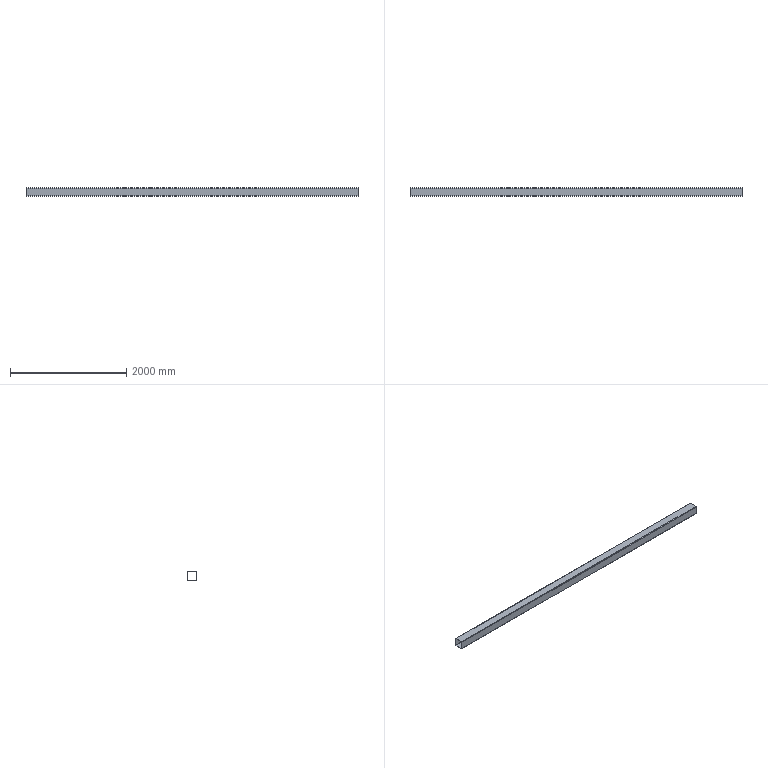Part | SolidWorks | features WeldMemberFeat 1, WeldmentFeature 1 | 1 solid | 18 faces | box 5700 x 150 x 150 mm | volume 16163031 mm3 | plane 10 | cylinder 8 | commonest cylinder face diameters 10 x4 20 x4
STEP:
#1=CARTESIAN_POINT('',(-2850.,75.,65.));
#2=VERTEX_POINT('',#1);
#3=CARTESIAN_POINT('',(-2850.,65.,75.));
#4=VERTEX_POINT('',#3);
#5=CARTESIAN_POINT('',(-2850.,65.,65.));
#6=DIRECTION('',(1.,0.,0.));
#7=DIRECTION('',(0.,1.,0.));
#8=AXIS2_PLACEMENT_3D('',#5,#6,#7);
#9=CIRCLE('',#8,10.);
#10=EDGE_CURVE('',#2,#4,#9,.T.);
#11=ORIENTED_EDGE('',*,*,#10,.T.);
#12=CARTESIAN_POINT('',(2850.,65.,75.));
#13=VERTEX_POINT('',#12);
#14=CARTESIAN_POINT('',(2850.,65.,75.));
#15=DIRECTION('',(-1.,0.,0.));
#16=VECTOR('',#15,1000.);
#17=LINE('',#14,#16);
#18=EDGE_CURVE('',#13,#4,#17,.T.);
#19=ORIENTED_EDGE('',*,*,#18,.F.);
#20=CARTESIAN_POINT('',(2850.,75.,65.));
#21=VERTEX_POINT('',#20);
#22=CARTESIAN_POINT('',(2850.,65.,65.));
#23=DIRECTION('',(1.,0.,0.));
#24=DIRECTION('',(0.,1.,0.));
#25=AXIS2_PLACEMENT_3D('',#22,#23,#24);
#26=CIRCLE('',#25,10.);
#27=EDGE_CURVE('',#21,#13,#26,.T.);
#28=ORIENTED_EDGE('',*,*,#27,.F.);
#29=CARTESIAN_POINT('',(2850.,75.,65.));
#30=DIRECTION('',(-1.,0.,0.));
#31=VECTOR('',#30,1000.);
#32=LINE('',#29,#31);
#33=EDGE_CURVE('',#21,#2,#32,.T.);
#34=ORIENTED_EDGE('',*,*,#33,.T.);
#35=EDGE_LOOP('',(#11,#19,#28,#34));
#36=FACE_OUTER_BOUND('',#35,.T.);
#37=CARTESIAN_POINT('',(2850.,65.,65.));
#38=DIRECTION('',(-1.,0.,0.));
#39=DIRECTION('',(0.,-1.,0.));
#40=AXIS2_PLACEMENT_3D('',#37,#38,#39);
#41=CYLINDRICAL_SURFACE('',#40,10.);
#42=ADVANCED_FACE('',(#36),#41,.T.);
#43=CARTESIAN_POINT('',(-2850.,-65.,75.));
#44=VERTEX_POINT('',#43);
#45=CARTESIAN_POINT('',(-2850.,65.,75.));
#46=DIRECTION('',(0.,-1.,0.));
#47=VECTOR('',#46,1000.);
#48=LINE('',#45,#47);
#49=EDGE_CURVE('',#4,#44,#48,.T.);
#50=ORIENTED_EDGE('',*,*,#49,.T.);
#51=CARTESIAN_POINT('',(2850.,-65.,75.));
#52=VERTEX_POINT('',#51);
#53=CARTESIAN_POINT('',(2850.,-65.,75.));
#54=DIRECTION('',(-1.,0.,0.));
#55=VECTOR('',#54,1000.);
#56=LINE('',#53,#55);
#57=EDGE_CURVE('',#52,#44,#56,.T.);
#58=ORIENTED_EDGE('',*,*,#57,.F.);
#59=CARTESIAN_POINT('',(2850.,65.,75.));
#60=DIRECTION('',(0.,-1.,0.));
#61=VECTOR('',#60,1000.);
#62=LINE('',#59,#61);
#63=EDGE_CURVE('',#13,#52,#62,.T.);
#64=ORIENTED_EDGE('',*,*,#63,.F.);
#65=ORIENTED_EDGE('',*,*,#18,.T.);
#66=EDGE_LOOP('',(#50,#58,#64,#65));
#67=FACE_OUTER_BOUND('',#66,.T.);
#68=CARTESIAN_POINT('',(2850.,65.,75.));
#69=DIRECTION('',(0.,0.,-1.));
#70=DIRECTION('',(-1.,0.,0.));
#71=AXIS2_PLACEMENT_3D('',#68,#69,#70);
#72=PLANE('',#71);
#73=ADVANCED_FACE('',(#67),#72,.F.);
#74=CARTESIAN_POINT('',(-2850.,-75.,65.));
#75=VERTEX_POINT('',#74);
#76=CARTESIAN_POINT('',(-2850.,-65.,65.));
#77=DIRECTION('',(1.,0.,0.));
#78=DIRECTION('',(0.,1.,0.));
#79=AXIS2_PLACEMENT_3D('',#76,#77,#78);
#80=CIRCLE('',#79,10.);
#81=EDGE_CURVE('',#44,#75,#80,.T.);
#82=ORIENTED_EDGE('',*,*,#81,.T.);
#83=CARTESIAN_POINT('',(2850.,-75.,65.));
#84=VERTEX_POINT('',#83);
#85=CARTESIAN_POINT('',(2850.,-75.,65.));
#86=DIRECTION('',(-1.,0.,0.));
#87=VECTOR('',#86,1000.);
#88=LINE('',#85,#87);
#89=EDGE_CURVE('',#84,#75,#88,.T.);
#90=ORIENTED_EDGE('',*,*,#89,.F.);
#91=CARTESIAN_POINT('',(2850.,-65.,65.));
#92=DIRECTION('',(1.,0.,0.));
#93=DIRECTION('',(0.,1.,0.));
#94=AXIS2_PLACEMENT_3D('',#91,#92,#93);
#95=CIRCLE('',#94,10.);
#96=EDGE_CURVE('',#52,#84,#95,.T.);
#97=ORIENTED_EDGE('',*,*,#96,.F.);
#98=ORIENTED_EDGE('',*,*,#57,.T.);
#99=EDGE_LOOP('',(#82,#90,#97,#98));
#100=FACE_OUTER_BOUND('',#99,.T.);
#101=CARTESIAN_POINT('',(2850.,-65.,65.));
#102=DIRECTION('',(-1.,0.,0.));
#103=DIRECTION('',(0.,-1.,0.));
#104=AXIS2_PLACEMENT_3D('',#101,#102,#103);
#105=CYLINDRICAL_SURFACE('',#104,10.);
#106=ADVANCED_FACE('',(#100),#105,.T.);
#107=CARTESIAN_POINT('',(-2850.,-75.,-65.));
#108=VERTEX_POINT('',#107);
#109=CARTESIAN_POINT('',(-2850.,-75.,-65.));
#110=DIRECTION('',(0.,0.,-1.));
#111=VECTOR('',#110,1000.);
#112=LINE('',#109,#111);
#113=EDGE_CURVE('',#75,#108,#112,.T.);
#114=ORIENTED_EDGE('',*,*,#113,.T.);
#115=CARTESIAN_POINT('',(2850.,-75.,-65.));
#116=VERTEX_POINT('',#115);
#117=CARTESIAN_POINT('',(2850.,-75.,-65.));
#118=DIRECTION('',(-1.,0.,0.));
#119=VECTOR('',#118,1000.);
#120=LINE('',#117,#119);
#121=EDGE_CURVE('',#116,#108,#120,.T.);
#122=ORIENTED_EDGE('',*,*,#121,.F.);
#123=CARTESIAN_POINT('',(2850.,-75.,-65.));
#124=DIRECTION('',(0.,0.,-1.));
#125=VECTOR('',#124,1000.);
#126=LINE('',#123,#125);
#127=EDGE_CURVE('',#84,#116,#126,.T.);
#128=ORIENTED_EDGE('',*,*,#127,.F.);
#129=ORIENTED_EDGE('',*,*,#89,.T.);
#130=EDGE_LOOP('',(#114,#122,#128,#129));
#131=FACE_OUTER_BOUND('',#130,.T.);
#132=CARTESIAN_POINT('',(2850.,-75.,-65.));
#133=DIRECTION('',(0.,1.,0.));
#134=DIRECTION('',(-1.,0.,0.));
#135=AXIS2_PLACEMENT_3D('',#132,#133,#134);
#136=PLANE('',#135);
#137=ADVANCED_FACE('',(#131),#136,.F.);
#138=CARTESIAN_POINT('',(-2850.,-65.,-75.));
#139=VERTEX_POINT('',#138);
#140=CARTESIAN_POINT('',(-2850.,-65.,-65.));
#141=DIRECTION('',(1.,0.,0.));
#142=DIRECTION('',(0.,1.,0.));
#143=AXIS2_PLACEMENT_3D('',#140,#141,#142);
#144=CIRCLE('',#143,10.);
#145=EDGE_CURVE('',#108,#139,#144,.T.);
#146=ORIENTED_EDGE('',*,*,#145,.T.);
#147=CARTESIAN_POINT('',(2850.,-65.,-75.));
#148=VERTEX_POINT('',#147);
#149=CARTESIAN_POINT('',(2850.,-65.,-75.));
#150=DIRECTION('',(-1.,0.,0.));
#151=VECTOR('',#150,1000.);
#152=LINE('',#149,#151);
#153=EDGE_CURVE('',#148,#139,#152,.T.);
#154=ORIENTED_EDGE('',*,*,#153,.F.);
#155=CARTESIAN_POINT('',(2850.,-65.,-65.));
#156=DIRECTION('',(1.,0.,0.));
#157=DIRECTION('',(0.,1.,0.));
#158=AXIS2_PLACEMENT_3D('',#155,#156,#157);
#159=CIRCLE('',#158,10.);
#160=EDGE_CURVE('',#116,#148,#159,.T.);
#161=ORIENTED_EDGE('',*,*,#160,.F.);
#162=ORIENTED_EDGE('',*,*,#121,.T.);
#163=EDGE_LOOP('',(#146,#154,#161,#162));
#164=FACE_OUTER_BOUND('',#163,.T.);
#165=CARTESIAN_POINT('',(2850.,-65.,-65.));
#166=DIRECTION('',(-1.,0.,0.));
#167=DIRECTION('',(0.,-1.,0.));
#168=AXIS2_PLACEMENT_3D('',#165,#166,#167);
#169=CYLINDRICAL_SURFACE('',#168,10.);
#170=ADVANCED_FACE('',(#164),#169,.T.);
#171=CARTESIAN_POINT('',(-2850.,65.,-75.));
#172=VERTEX_POINT('',#171);
#173=CARTESIAN_POINT('',(-2850.,-65.,-75.));
#174=DIRECTION('',(0.,1.,0.));
#175=VECTOR('',#174,1000.);
#176=LINE('',#173,#175);
#177=EDGE_CURVE('',#139,#172,#176,.T.);
#178=ORIENTED_EDGE('',*,*,#177,.T.);
#179=CARTESIAN_POINT('',(2850.,65.,-75.));
#180=VERTEX_POINT('',#179);
#181=CARTESIAN_POINT('',(2850.,65.,-75.));
#182=DIRECTION('',(-1.,0.,0.));
#183=VECTOR('',#182,1000.);
#184=LINE('',#181,#183);
#185=EDGE_CURVE('',#180,#172,#184,.T.);
#186=ORIENTED_EDGE('',*,*,#185,.F.);
#187=CARTESIAN_POINT('',(2850.,-65.,-75.));
#188=DIRECTION('',(0.,1.,0.));
#189=VECTOR('',#188,1000.);
#190=LINE('',#187,#189);
#191=EDGE_CURVE('',#148,#180,#190,.T.);
#192=ORIENTED_EDGE('',*,*,#191,.F.);
#193=ORIENTED_EDGE('',*,*,#153,.T.);
#194=EDGE_LOOP('',(#178,#186,#192,#193));
#195=FACE_OUTER_BOUND('',#194,.T.);
#196=CARTESIAN_POINT('',(2850.,-65.,-75.));
#197=DIRECTION('',(0.,0.,1.));
#198=DIRECTION('',(1.,0.,0.));
#199=AXIS2_PLACEMENT_3D('',#196,#197,#198);
#200=PLANE('',#199);
#201=ADVANCED_FACE('',(#195),#200,.F.);
#202=CARTESIAN_POINT('',(-2850.,75.,-65.));
#203=VERTEX_POINT('',#202);
#204=CARTESIAN_POINT('',(-2850.,65.,-65.));
#205=DIRECTION('',(1.,0.,0.));
#206=DIRECTION('',(0.,1.,0.));
#207=AXIS2_PLACEMENT_3D('',#204,#205,#206);
#208=CIRCLE('',#207,10.);
#209=EDGE_CURVE('',#172,#203,#208,.T.);
#210=ORIENTED_EDGE('',*,*,#209,.T.);
#211=CARTESIAN_POINT('',(2850.,75.,-65.));
#212=VERTEX_POINT('',#211);
#213=CARTESIAN_POINT('',(2850.,75.,-65.));
#214=DIRECTION('',(-1.,0.,0.));
#215=VECTOR('',#214,1000.);
#216=LINE('',#213,#215);
#217=EDGE_CURVE('',#212,#203,#216,.T.);
#218=ORIENTED_EDGE('',*,*,#217,.F.);
#219=CARTESIAN_POINT('',(2850.,65.,-65.));
#220=DIRECTION('',(1.,0.,0.));
#221=DIRECTION('',(0.,1.,0.));
#222=AXIS2_PLACEMENT_3D('',#219,#220,#221);
#223=CIRCLE('',#222,10.);
#224=EDGE_CURVE('',#180,#212,#223,.T.);
#225=ORIENTED_EDGE('',*,*,#224,.F.);
#226=ORIENTED_EDGE('',*,*,#185,.T.);
#227=EDGE_LOOP('',(#210,#218,#225,#226));
#228=FACE_OUTER_BOUND('',#227,.T.);
#229=CARTESIAN_POINT('',(2850.,65.,-65.));
#230=DIRECTION('',(-1.,0.,0.));
#231=DIRECTION('',(0.,-1.,0.));
#232=AXIS2_PLACEMENT_3D('',#229,#230,#231);
#233=CYLINDRICAL_SURFACE('',#232,10.);
#234=ADVANCED_FACE('',(#228),#233,.T.);
#235=CARTESIAN_POINT('',(-2850.,-65.,70.));
#236=VERTEX_POINT('',#235);
#237=CARTESIAN_POINT('',(-2850.,-70.,65.));
#238=VERTEX_POINT('',#237);
#239=CARTESIAN_POINT('',(-2850.,-65.,65.));
#240=DIRECTION('',(1.,0.,0.));
#241=DIRECTION('',(0.,1.,0.));
#242=AXIS2_PLACEMENT_3D('',#239,#240,#241);
#243=CIRCLE('',#242,5.);
#244=EDGE_CURVE('',#236,#238,#243,.T.);
#245=ORIENTED_EDGE('',*,*,#244,.F.);
#246=CARTESIAN_POINT('',(2850.,-65.,70.));
#247=VERTEX_POINT('',#246);
#248=CARTESIAN_POINT('',(2850.,-65.,70.));
#249=DIRECTION('',(-1.,0.,0.));
#250=VECTOR('',#249,1000.);
#251=LINE('',#248,#250);
#252=EDGE_CURVE('',#247,#236,#251,.T.);
#253=ORIENTED_EDGE('',*,*,#252,.F.);
#254=CARTESIAN_POINT('',(2850.,-70.,65.));
#255=VERTEX_POINT('',#254);
#256=CARTESIAN_POINT('',(2850.,-65.,65.));
#257=DIRECTION('',(1.,0.,0.));
#258=DIRECTION('',(0.,1.,0.));
#259=AXIS2_PLACEMENT_3D('',#256,#257,#258);
#260=CIRCLE('',#259,5.);
#261=EDGE_CURVE('',#247,#255,#260,.T.);
#262=ORIENTED_EDGE('',*,*,#261,.T.);
#263=CARTESIAN_POINT('',(2850.,-70.,65.));
#264=DIRECTION('',(-1.,0.,0.));
#265=VECTOR('',#264,1000.);
#266=LINE('',#263,#265);
#267=EDGE_CURVE('',#255,#238,#266,.T.);
#268=ORIENTED_EDGE('',*,*,#267,.T.);
#269=EDGE_LOOP('',(#245,#253,#262,#268));
#270=FACE_OUTER_BOUND('',#269,.T.);
#271=CARTESIAN_POINT('',(2850.,-65.,65.));
#272=DIRECTION('',(-1.,0.,0.));
#273=DIRECTION('',(0.,-1.,0.));
#274=AXIS2_PLACEMENT_3D('',#271,#272,#273);
#275=CYLINDRICAL_SURFACE('',#274,5.);
#276=ADVANCED_FACE('',(#270),#275,.F.);
#277=CARTESIAN_POINT('',(-2850.,65.,70.));
#278=VERTEX_POINT('',#277);
#279=CARTESIAN_POINT('',(-2850.,65.,70.));
#280=DIRECTION('',(0.,-1.,0.));
#281=VECTOR('',#280,1000.);
#282=LINE('',#279,#281);
#283=EDGE_CURVE('',#278,#236,#282,.T.);
#284=ORIENTED_EDGE('',*,*,#283,.F.);
#285=CARTESIAN_POINT('',(2850.,65.,70.));
#286=VERTEX_POINT('',#285);
#287=CARTESIAN_POINT('',(2850.,65.,70.));
#288=DIRECTION('',(-1.,0.,0.));
#289=VECTOR('',#288,1000.);
#290=LINE('',#287,#289);
#291=EDGE_CURVE('',#286,#278,#290,.T.);
#292=ORIENTED_EDGE('',*,*,#291,.F.);
#293=CARTESIAN_POINT('',(2850.,65.,70.));
#294=DIRECTION('',(0.,-1.,0.));
#295=VECTOR('',#294,1000.);
#296=LINE('',#293,#295);
#297=EDGE_CURVE('',#286,#247,#296,.T.);
#298=ORIENTED_EDGE('',*,*,#297,.T.);
#299=ORIENTED_EDGE('',*,*,#252,.T.);
#300=EDGE_LOOP('',(#284,#292,#298,#299));
#301=FACE_OUTER_BOUND('',#300,.T.);
#302=CARTESIAN_POINT('',(2850.,65.,70.));
#303=DIRECTION('',(0.,0.,-1.));
#304=DIRECTION('',(-1.,0.,0.));
#305=AXIS2_PLACEMENT_3D('',#302,#303,#304);
#306=PLANE('',#305);
#307=ADVANCED_FACE('',(#301),#306,.T.);
#308=CARTESIAN_POINT('',(-2850.,70.,65.));
#309=VERTEX_POINT('',#308);
#310=CARTESIAN_POINT('',(-2850.,65.,65.));
#311=DIRECTION('',(1.,0.,0.));
#312=DIRECTION('',(0.,1.,0.));
#313=AXIS2_PLACEMENT_3D('',#310,#311,#312);
#314=CIRCLE('',#313,5.);
#315=EDGE_CURVE('',#309,#278,#314,.T.);
#316=ORIENTED_EDGE('',*,*,#315,.F.);
#317=CARTESIAN_POINT('',(2850.,70.,65.));
#318=VERTEX_POINT('',#317);
#319=CARTESIAN_POINT('',(2850.,70.,65.));
#320=DIRECTION('',(-1.,0.,0.));
#321=VECTOR('',#320,1000.);
#322=LINE('',#319,#321);
#323=EDGE_CURVE('',#318,#309,#322,.T.);
#324=ORIENTED_EDGE('',*,*,#323,.F.);
#325=CARTESIAN_POINT('',(2850.,65.,65.));
#326=DIRECTION('',(1.,0.,0.));
#327=DIRECTION('',(0.,1.,0.));
#328=AXIS2_PLACEMENT_3D('',#325,#326,#327);
#329=CIRCLE('',#328,5.);
#330=EDGE_CURVE('',#318,#286,#329,.T.);
#331=ORIENTED_EDGE('',*,*,#330,.T.);
#332=ORIENTED_EDGE('',*,*,#291,.T.);
#333=EDGE_LOOP('',(#316,#324,#331,#332));
#334=FACE_OUTER_BOUND('',#333,.T.);
#335=CARTESIAN_POINT('',(2850.,65.,65.));
#336=DIRECTION('',(-1.,0.,0.));
#337=DIRECTION('',(0.,-1.,0.));
#338=AXIS2_PLACEMENT_3D('',#335,#336,#337);
#339=CYLINDRICAL_SURFACE('',#338,5.);
#340=ADVANCED_FACE('',(#334),#339,.F.);
#341=CARTESIAN_POINT('',(-2850.,70.,-65.));
#342=VERTEX_POINT('',#341);
#343=CARTESIAN_POINT('',(-2850.,70.,65.));
#344=DIRECTION('',(0.,0.,1.));
#345=VECTOR('',#344,1000.);
#346=LINE('',#343,#345);
#347=EDGE_CURVE('',#342,#309,#346,.T.);
#348=ORIENTED_EDGE('',*,*,#347,.F.);
#349=CARTESIAN_POINT('',(2850.,70.,-65.));
#350=VERTEX_POINT('',#349);
#351=CARTESIAN_POINT('',(2850.,70.,-65.));
#352=DIRECTION('',(-1.,0.,0.));
#353=VECTOR('',#352,1000.);
#354=LINE('',#351,#353);
#355=EDGE_CURVE('',#350,#342,#354,.T.);
#356=ORIENTED_EDGE('',*,*,#355,.F.);
#357=CARTESIAN_POINT('',(2850.,70.,65.));
#358=DIRECTION('',(0.,0.,1.));
#359=VECTOR('',#358,1000.);
#360=LINE('',#357,#359);
#361=EDGE_CURVE('',#350,#318,#360,.T.);
#362=ORIENTED_EDGE('',*,*,#361,.T.);
#363=ORIENTED_EDGE('',*,*,#323,.T.);
#364=EDGE_LOOP('',(#348,#356,#362,#363));
#365=FACE_OUTER_BOUND('',#364,.T.);
#366=CARTESIAN_POINT('',(2850.,70.,65.));
#367=DIRECTION('',(0.,-1.,0.));
#368=DIRECTION('',(1.,0.,0.));
#369=AXIS2_PLACEMENT_3D('',#366,#367,#368);
#370=PLANE('',#369);
#371=ADVANCED_FACE('',(#365),#370,.T.);
#372=CARTESIAN_POINT('',(-2850.,65.,-70.));
#373=VERTEX_POINT('',#372);
#374=CARTESIAN_POINT('',(-2850.,65.,-65.));
#375=DIRECTION('',(1.,0.,0.));
#376=DIRECTION('',(0.,1.,0.));
#377=AXIS2_PLACEMENT_3D('',#374,#375,#376);
#378=CIRCLE('',#377,5.);
#379=EDGE_CURVE('',#373,#342,#378,.T.);
#380=ORIENTED_EDGE('',*,*,#379,.F.);
#381=CARTESIAN_POINT('',(2850.,65.,-70.));
#382=VERTEX_POINT('',#381);
#383=CARTESIAN_POINT('',(2850.,65.,-70.));
#384=DIRECTION('',(-1.,0.,0.));
#385=VECTOR('',#384,1000.);
#386=LINE('',#383,#385);
#387=EDGE_CURVE('',#382,#373,#386,.T.);
#388=ORIENTED_EDGE('',*,*,#387,.F.);
#389=CARTESIAN_POINT('',(2850.,65.,-65.));
#390=DIRECTION('',(1.,0.,0.));
#391=DIRECTION('',(0.,1.,0.));
#392=AXIS2_PLACEMENT_3D('',#389,#390,#391);
#393=CIRCLE('',#392,5.);
#394=EDGE_CURVE('',#382,#350,#393,.T.);
#395=ORIENTED_EDGE('',*,*,#394,.T.);
#396=ORIENTED_EDGE('',*,*,#355,.T.);
#397=EDGE_LOOP('',(#380,#388,#395,#396));
#398=FACE_OUTER_BOUND('',#397,.T.);
#399=CARTESIAN_POINT('',(2850.,65.,-65.));
#400=DIRECTION('',(-1.,0.,0.));
#401=DIRECTION('',(0.,-1.,0.));
#402=AXIS2_PLACEMENT_3D('',#399,#400,#401);
#403=CYLINDRICAL_SURFACE('',#402,5.);
#404=ADVANCED_FACE('',(#398),#403,.F.);
#405=CARTESIAN_POINT('',(-2850.,-65.,-70.));
#406=VERTEX_POINT('',#405);
#407=CARTESIAN_POINT('',(-2850.,-65.,-70.));
#408=DIRECTION('',(0.,1.,0.));
#409=VECTOR('',#408,1000.);
#410=LINE('',#407,#409);
#411=EDGE_CURVE('',#406,#373,#410,.T.);
#412=ORIENTED_EDGE('',*,*,#411,.F.);
#413=CARTESIAN_POINT('',(2850.,-65.,-70.));
#414=VERTEX_POINT('',#413);
#415=CARTESIAN_POINT('',(2850.,-65.,-70.));
#416=DIRECTION('',(-1.,0.,0.));
#417=VECTOR('',#416,1000.);
#418=LINE('',#415,#417);
#419=EDGE_CURVE('',#414,#406,#418,.T.);
#420=ORIENTED_EDGE('',*,*,#419,.F.);
#421=CARTESIAN_POINT('',(2850.,-65.,-70.));
#422=DIRECTION('',(0.,1.,0.));
#423=VECTOR('',#422,1000.);
#424=LINE('',#421,#423);
#425=EDGE_CURVE('',#414,#382,#424,.T.);
#426=ORIENTED_EDGE('',*,*,#425,.T.);
#427=ORIENTED_EDGE('',*,*,#387,.T.);
#428=EDGE_LOOP('',(#412,#420,#426,#427));
#429=FACE_OUTER_BOUND('',#428,.T.);
#430=CARTESIAN_POINT('',(2850.,-65.,-70.));
#431=DIRECTION('',(0.,0.,1.));
#432=DIRECTION('',(1.,0.,0.));
#433=AXIS2_PLACEMENT_3D('',#430,#431,#432);
#434=PLANE('',#433);
#435=ADVANCED_FACE('',(#429),#434,.T.);
#436=CARTESIAN_POINT('',(-2850.,-70.,-65.));
#437=VERTEX_POINT('',#436);
#438=CARTESIAN_POINT('',(-2850.,-65.,-65.));
#439=DIRECTION('',(1.,0.,0.));
#440=DIRECTION('',(0.,1.,0.));
#441=AXIS2_PLACEMENT_3D('',#438,#439,#440);
#442=CIRCLE('',#441,5.);
#443=EDGE_CURVE('',#437,#406,#442,.T.);
#444=ORIENTED_EDGE('',*,*,#443,.F.);
#445=CARTESIAN_POINT('',(2850.,-70.,-65.));
#446=VERTEX_POINT('',#445);
#447=CARTESIAN_POINT('',(2850.,-70.,-65.));
#448=DIRECTION('',(-1.,0.,0.));
#449=VECTOR('',#448,1000.);
#450=LINE('',#447,#449);
#451=EDGE_CURVE('',#446,#437,#450,.T.);
#452=ORIENTED_EDGE('',*,*,#451,.F.);
#453=CARTESIAN_POINT('',(2850.,-65.,-65.));
#454=DIRECTION('',(1.,0.,0.));
#455=DIRECTION('',(0.,1.,0.));
#456=AXIS2_PLACEMENT_3D('',#453,#454,#455);
#457=CIRCLE('',#456,5.);
#458=EDGE_CURVE('',#446,#414,#457,.T.);
#459=ORIENTED_EDGE('',*,*,#458,.T.);
#460=ORIENTED_EDGE('',*,*,#419,.T.);
#461=EDGE_LOOP('',(#444,#452,#459,#460));
#462=FACE_OUTER_BOUND('',#461,.T.);
#463=CARTESIAN_POINT('',(2850.,-65.,-65.));
#464=DIRECTION('',(-1.,0.,0.));
#465=DIRECTION('',(0.,-1.,0.));
#466=AXIS2_PLACEMENT_3D('',#463,#464,#465);
#467=CYLINDRICAL_SURFACE('',#466,5.);
#468=ADVANCED_FACE('',(#462),#467,.F.);
#469=CARTESIAN_POINT('',(-2850.,-70.,-65.));
#470=DIRECTION('',(0.,0.,-1.));
#471=VECTOR('',#470,1000.);
#472=LINE('',#469,#471);
#473=EDGE_CURVE('',#238,#437,#472,.T.);
#474=ORIENTED_EDGE('',*,*,#473,.F.);
#475=ORIENTED_EDGE('',*,*,#267,.F.);
#476=CARTESIAN_POINT('',(2850.,-70.,-65.));
#477=DIRECTION('',(0.,0.,-1.));
#478=VECTOR('',#477,1000.);
#479=LINE('',#476,#478);
#480=EDGE_CURVE('',#255,#446,#479,.T.);
#481=ORIENTED_EDGE('',*,*,#480,.T.);
#482=ORIENTED_EDGE('',*,*,#451,.T.);
#483=EDGE_LOOP('',(#474,#475,#481,#482));
#484=FACE_OUTER_BOUND('',#483,.T.);
#485=CARTESIAN_POINT('',(2850.,-70.,-65.));
#486=DIRECTION('',(0.,1.,0.));
#487=DIRECTION('',(-1.,0.,0.));
#488=AXIS2_PLACEMENT_3D('',#485,#486,#487);
#489=PLANE('',#488);
#490=ADVANCED_FACE('',(#484),#489,.T.);
#491=CARTESIAN_POINT('',(-2850.,75.,65.));
#492=DIRECTION('',(0.,0.,1.));
#493=VECTOR('',#492,1000.);
#494=LINE('',#491,#493);
#495=EDGE_CURVE('',#203,#2,#494,.T.);
#496=ORIENTED_EDGE('',*,*,#495,.T.);
#497=ORIENTED_EDGE('',*,*,#33,.F.);
#498=CARTESIAN_POINT('',(2850.,75.,65.));
#499=DIRECTION('',(0.,0.,1.));
#500=VECTOR('',#499,1000.);
#501=LINE('',#498,#500);
#502=EDGE_CURVE('',#212,#21,#501,.T.);
#503=ORIENTED_EDGE('',*,*,#502,.F.);
#504=ORIENTED_EDGE('',*,*,#217,.T.);
#505=EDGE_LOOP('',(#496,#497,#503,#504));
#506=FACE_OUTER_BOUND('',#505,.T.);
#507=CARTESIAN_POINT('',(2850.,75.,65.));
#508=DIRECTION('',(0.,-1.,0.));
#509=DIRECTION('',(1.,0.,0.));
#510=AXIS2_PLACEMENT_3D('',#507,#508,#509);
#511=PLANE('',#510);
#512=ADVANCED_FACE('',(#506),#511,.F.);
#513=ORIENTED_EDGE('',*,*,#261,.F.);
#514=ORIENTED_EDGE('',*,*,#297,.F.);
#515=ORIENTED_EDGE('',*,*,#330,.F.);
#516=ORIENTED_EDGE('',*,*,#361,.F.);
#517=ORIENTED_EDGE('',*,*,#394,.F.);
#518=ORIENTED_EDGE('',*,*,#425,.F.);
#519=ORIENTED_EDGE('',*,*,#458,.F.);
#520=ORIENTED_EDGE('',*,*,#480,.F.);
#521=EDGE_LOOP('',(#513,#514,#515,#516,#517,#518,#519,#520));
#522=FACE_BOUND('',#521,.T.);
#523=ORIENTED_EDGE('',*,*,#27,.T.);
#524=ORIENTED_EDGE('',*,*,#63,.T.);
#525=ORIENTED_EDGE('',*,*,#96,.T.);
#526=ORIENTED_EDGE('',*,*,#127,.T.);
#527=ORIENTED_EDGE('',*,*,#160,.T.);
#528=ORIENTED_EDGE('',*,*,#191,.T.);
#529=ORIENTED_EDGE('',*,*,#224,.T.);
#530=ORIENTED_EDGE('',*,*,#502,.T.);
#531=EDGE_LOOP('',(#523,#524,#525,#526,#527,#528,#529,#530));
#532=FACE_OUTER_BOUND('',#531,.T.);
#533=CARTESIAN_POINT('',(2850.,65.,65.));
#534=DIRECTION('',(1.,0.,0.));
#535=DIRECTION('',(0.,1.,0.));
#536=AXIS2_PLACEMENT_3D('',#533,#534,#535);
#537=PLANE('',#536);
#538=ADVANCED_FACE('',(#522,#532),#537,.T.);
#539=ORIENTED_EDGE('',*,*,#244,.T.);
#540=ORIENTED_EDGE('',*,*,#473,.T.);
#541=ORIENTED_EDGE('',*,*,#443,.T.);
#542=ORIENTED_EDGE('',*,*,#411,.T.);
#543=ORIENTED_EDGE('',*,*,#379,.T.);
#544=ORIENTED_EDGE('',*,*,#347,.T.);
#545=ORIENTED_EDGE('',*,*,#315,.T.);
#546=ORIENTED_EDGE('',*,*,#283,.T.);
#547=EDGE_LOOP('',(#539,#540,#541,#542,#543,#544,#545,#546));
#548=FACE_BOUND('',#547,.T.);
#549=ORIENTED_EDGE('',*,*,#10,.F.);
#550=ORIENTED_EDGE('',*,*,#495,.F.);
#551=ORIENTED_EDGE('',*,*,#209,.F.);
#552=ORIENTED_EDGE('',*,*,#177,.F.);
#553=ORIENTED_EDGE('',*,*,#145,.F.);
#554=ORIENTED_EDGE('',*,*,#113,.F.);
#555=ORIENTED_EDGE('',*,*,#81,.F.);
#556=ORIENTED_EDGE('',*,*,#49,.F.);
#557=EDGE_LOOP('',(#549,#550,#551,#552,#553,#554,#555,#556));
#558=FACE_OUTER_BOUND('',#557,.T.);
#559=CARTESIAN_POINT('',(-2850.,65.,65.));
#560=DIRECTION('',(1.,0.,0.));
#561=DIRECTION('',(0.,1.,0.));
#562=AXIS2_PLACEMENT_3D('',#559,#560,#561);
#563=PLANE('',#562);
#564=ADVANCED_FACE('',(#548,#558),#563,.F.);
#565=CLOSED_SHELL('',(#42,#73,#106,#137,#170,#201,#234,#276,#307,#340,#371,#404,#435,#468,#490,#512,#538,#564));
#566=MANIFOLD_SOLID_BREP('',#565);
#567=CARTESIAN_POINT('',(0.,0.,0.));
#568=DIRECTION('',(0.,0.,1.));
#569=DIRECTION('',(1.,0.,0.));
#570=AXIS2_PLACEMENT_3D('',#567,#568,#569);
#571=(LENGTH_UNIT()NAMED_UNIT(*)SI_UNIT(.MILLI.,.METRE.));
#572=UNCERTAINTY_MEASURE_WITH_UNIT(LENGTH_MEASURE(0.00001),#571,'','');
#573=(NAMED_UNIT(*)PLANE_ANGLE_UNIT()SI_UNIT($,.RADIAN.));
#574=(NAMED_UNIT(*)SI_UNIT($,.STERADIAN.)SOLID_ANGLE_UNIT());
#575=(GEOMETRIC_REPRESENTATION_CONTEXT(3)GLOBAL_UNCERTAINTY_ASSIGNED_CONTEXT((#572))GLOBAL_UNIT_ASSIGNED_CONTEXT((#571,#573,#574))REPRESENTATION_CONTEXT('',''));
#576=ADVANCED_BREP_SHAPE_REPRESENTATION('',(#566,#570),#575);